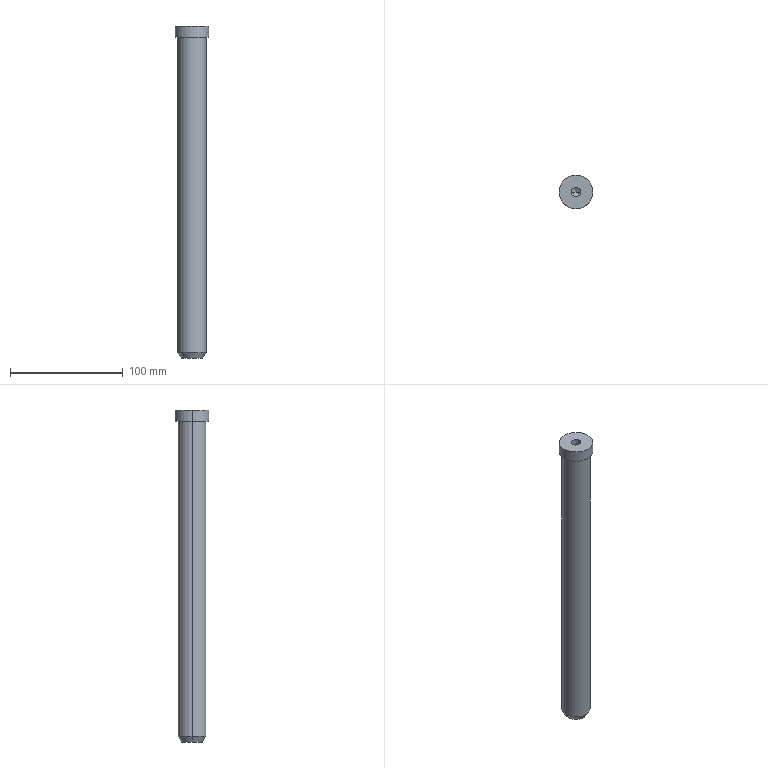Part | Creo | 1 solid | 13 faces | box 30 x 30 x 295 mm | volume 145243 mm3 | cylinder 6 | cone 4 | plane 3 | commonest cylinder face diameters 8.5 x2 25 x2 30 x2
STEP:
#1=CARTESIAN_POINT('',(0.,0.,0.));
#2=DIRECTION('',(0.,0.,1.));
#3=DIRECTION('',(1.,0.,0.));
#4=AXIS2_PLACEMENT_3D('',#1,#2,#3);
#5=CARTESIAN_POINT('',(-153.,131.,300.5));
#6=VERTEX_POINT('',#5);
#7=CARTESIAN_POINT('',(-123.,131.,300.5));
#8=VERTEX_POINT('',#7);
#9=CARTESIAN_POINT('',(-138.,131.,300.5));
#10=DIRECTION('',(0.,0.,-1.));
#11=DIRECTION('',(-1.,0.,0.));
#12=AXIS2_PLACEMENT_3D('',#9,#10,#11);
#13=CIRCLE('',#12,15.);
#14=EDGE_CURVE('',#6,#8,#13,.T.);
#15=ORIENTED_EDGE('',*,*,#14,.F.);
#16=CARTESIAN_POINT('',(-138.,131.,300.5));
#17=DIRECTION('',(0.,0.,-1.));
#18=DIRECTION('',(1.,0.,0.));
#19=AXIS2_PLACEMENT_3D('',#16,#17,#18);
#20=CIRCLE('',#19,15.);
#21=EDGE_CURVE('',#8,#6,#20,.T.);
#22=ORIENTED_EDGE('',*,*,#21,.F.);
#23=EDGE_LOOP('',(#15,#22));
#24=FACE_OUTER_BOUND('',#23,.F.);
#25=CARTESIAN_POINT('',(-150.5,131.,300.5));
#26=VERTEX_POINT('',#25);
#27=CARTESIAN_POINT('',(-125.5,131.,300.5));
#28=VERTEX_POINT('',#27);
#29=CARTESIAN_POINT('',(-138.,131.,300.5));
#30=DIRECTION('',(0.,0.,1.));
#31=DIRECTION('',(-1.,0.,0.));
#32=AXIS2_PLACEMENT_3D('',#29,#30,#31);
#33=CIRCLE('',#32,12.5);
#34=EDGE_CURVE('',#26,#28,#33,.T.);
#35=ORIENTED_EDGE('',*,*,#34,.F.);
#36=CARTESIAN_POINT('',(-138.,131.,300.5));
#37=DIRECTION('',(0.,0.,1.));
#38=DIRECTION('',(1.,0.,0.));
#39=AXIS2_PLACEMENT_3D('',#36,#37,#38);
#40=CIRCLE('',#39,12.5);
#41=EDGE_CURVE('',#28,#26,#40,.T.);
#42=ORIENTED_EDGE('',*,*,#41,.F.);
#43=EDGE_LOOP('',(#35,#42));
#44=FACE_BOUND('',#43,.F.);
#45=CARTESIAN_POINT('',(-138.,131.,300.5));
#46=DIRECTION('',(0.,0.,-1.));
#47=DIRECTION('',(-1.,0.,0.));
#48=AXIS2_PLACEMENT_3D('',#45,#46,#47);
#49=PLANE('',#48);
#50=ADVANCED_FACE('',(#24,#44),#49,.T.);
#51=CARTESIAN_POINT('',(-125.5,131.,20.5));
#52=VERTEX_POINT('',#51);
#53=CARTESIAN_POINT('',(-150.5,131.,20.5));
#54=VERTEX_POINT('',#53);
#55=CARTESIAN_POINT('',(-138.,131.,20.5));
#56=DIRECTION('',(0.,0.,-1.));
#57=DIRECTION('',(1.,0.,0.));
#58=AXIS2_PLACEMENT_3D('',#55,#56,#57);
#59=CIRCLE('',#58,12.5);
#60=EDGE_CURVE('',#52,#54,#59,.T.);
#61=ORIENTED_EDGE('',*,*,#60,.T.);
#62=CARTESIAN_POINT('',(-150.5,131.,20.5));
#63=DIRECTION('',(0.,0.,1.));
#64=VECTOR('',#63,280.);
#65=LINE('',#62,#64);
#66=EDGE_CURVE('',#54,#26,#65,.T.);
#67=ORIENTED_EDGE('',*,*,#66,.T.);
#68=ORIENTED_EDGE('',*,*,#34,.T.);
#69=CARTESIAN_POINT('',(-125.5,131.,20.5));
#70=DIRECTION('',(0.,0.,1.));
#71=VECTOR('',#70,280.);
#72=LINE('',#69,#71);
#73=EDGE_CURVE('',#52,#28,#72,.T.);
#74=ORIENTED_EDGE('',*,*,#73,.F.);
#75=EDGE_LOOP('',(#61,#67,#68,#74));
#76=FACE_OUTER_BOUND('',#75,.F.);
#77=CARTESIAN_POINT('',(-138.,131.,10.5));
#78=DIRECTION('',(0.,0.,1.));
#79=DIRECTION('',(1.,0.,0.));
#80=AXIS2_PLACEMENT_3D('',#77,#78,#79);
#81=CYLINDRICAL_SURFACE('',#80,12.5);
#82=ADVANCED_FACE('',(#76),#81,.T.);
#83=CARTESIAN_POINT('',(-128.5,131.,15.5));
#84=VERTEX_POINT('',#83);
#85=CARTESIAN_POINT('',(-147.5,131.,15.5));
#86=VERTEX_POINT('',#85);
#87=CARTESIAN_POINT('',(-138.,131.,15.5));
#88=DIRECTION('',(0.,0.,-1.));
#89=DIRECTION('',(1.,0.,0.));
#90=AXIS2_PLACEMENT_3D('',#87,#88,#89);
#91=CIRCLE('',#90,9.5);
#92=EDGE_CURVE('',#84,#86,#91,.T.);
#93=ORIENTED_EDGE('',*,*,#92,.T.);
#94=CARTESIAN_POINT('',(-147.5,131.,15.5));
#95=DIRECTION('',(-0.5145,0.,0.8575));
#96=VECTOR('',#95,5.831);
#97=LINE('',#94,#96);
#98=EDGE_CURVE('',#86,#54,#97,.T.);
#99=ORIENTED_EDGE('',*,*,#98,.T.);
#100=ORIENTED_EDGE('',*,*,#60,.F.);
#101=CARTESIAN_POINT('',(-128.5,131.,15.5));
#102=DIRECTION('',(0.5145,0.,0.8575));
#103=VECTOR('',#102,5.831);
#104=LINE('',#101,#103);
#105=EDGE_CURVE('',#84,#52,#104,.T.);
#106=ORIENTED_EDGE('',*,*,#105,.F.);
#107=EDGE_LOOP('',(#93,#99,#100,#106));
#108=FACE_OUTER_BOUND('',#107,.F.);
#109=CARTESIAN_POINT('',(-138.,131.,18.));
#110=DIRECTION('',(0.,0.,1.));
#111=DIRECTION('',(1.,0.,0.));
#112=AXIS2_PLACEMENT_3D('',#109,#110,#111);
#113=CONICAL_SURFACE('',#112,11.,30.964);
#114=ADVANCED_FACE('',(#108),#113,.T.);
#115=ORIENTED_EDGE('',*,*,#92,.F.);
#116=CARTESIAN_POINT('',(-138.,131.,15.5));
#117=DIRECTION('',(0.,0.,-1.));
#118=DIRECTION('',(-1.,0.,0.));
#119=AXIS2_PLACEMENT_3D('',#116,#117,#118);
#120=CIRCLE('',#119,9.5);
#121=EDGE_CURVE('',#86,#84,#120,.T.);
#122=ORIENTED_EDGE('',*,*,#121,.F.);
#123=EDGE_LOOP('',(#115,#122));
#124=FACE_OUTER_BOUND('',#123,.F.);
#125=CARTESIAN_POINT('',(-138.,131.,15.5));
#126=DIRECTION('',(0.,0.,1.));
#127=DIRECTION('',(1.,0.,0.));
#128=AXIS2_PLACEMENT_3D('',#125,#126,#127);
#129=PLANE('',#128);
#130=ADVANCED_FACE('',(#124),#129,.F.);
#131=ORIENTED_EDGE('',*,*,#121,.T.);
#132=ORIENTED_EDGE('',*,*,#105,.T.);
#133=CARTESIAN_POINT('',(-138.,131.,20.5));
#134=DIRECTION('',(0.,0.,-1.));
#135=DIRECTION('',(-1.,0.,0.));
#136=AXIS2_PLACEMENT_3D('',#133,#134,#135);
#137=CIRCLE('',#136,12.5);
#138=EDGE_CURVE('',#54,#52,#137,.T.);
#139=ORIENTED_EDGE('',*,*,#138,.F.);
#140=ORIENTED_EDGE('',*,*,#98,.F.);
#141=EDGE_LOOP('',(#131,#132,#139,#140));
#142=FACE_OUTER_BOUND('',#141,.F.);
#143=CARTESIAN_POINT('',(-138.,131.,18.));
#144=DIRECTION('',(0.,0.,1.));
#145=DIRECTION('',(1.,0.,0.));
#146=AXIS2_PLACEMENT_3D('',#143,#144,#145);
#147=CONICAL_SURFACE('',#146,11.,30.964);
#148=ADVANCED_FACE('',(#142),#147,.T.);
#149=ORIENTED_EDGE('',*,*,#138,.T.);
#150=ORIENTED_EDGE('',*,*,#73,.T.);
#151=ORIENTED_EDGE('',*,*,#41,.T.);
#152=ORIENTED_EDGE('',*,*,#66,.F.);
#153=EDGE_LOOP('',(#149,#150,#151,#152));
#154=FACE_OUTER_BOUND('',#153,.F.);
#155=CARTESIAN_POINT('',(-138.,131.,10.5));
#156=DIRECTION('',(0.,0.,1.));
#157=DIRECTION('',(1.,0.,0.));
#158=AXIS2_PLACEMENT_3D('',#155,#156,#157);
#159=CYLINDRICAL_SURFACE('',#158,12.5);
#160=ADVANCED_FACE('',(#154),#159,.T.);
#161=ORIENTED_EDGE('',*,*,#14,.T.);
#162=CARTESIAN_POINT('',(-123.,131.,310.5));
#163=VERTEX_POINT('',#162);
#164=CARTESIAN_POINT('',(-123.,131.,310.5));
#165=DIRECTION('',(0.,0.,-1.));
#166=VECTOR('',#165,10.);
#167=LINE('',#164,#166);
#168=EDGE_CURVE('',#163,#8,#167,.T.);
#169=ORIENTED_EDGE('',*,*,#168,.F.);
#170=CARTESIAN_POINT('',(-153.,131.,310.5));
#171=VERTEX_POINT('',#170);
#172=CARTESIAN_POINT('',(-138.,131.,310.5));
#173=DIRECTION('',(0.,0.,1.));
#174=DIRECTION('',(1.,0.,0.));
#175=AXIS2_PLACEMENT_3D('',#172,#173,#174);
#176=CIRCLE('',#175,15.);
#177=EDGE_CURVE('',#163,#171,#176,.T.);
#178=ORIENTED_EDGE('',*,*,#177,.T.);
#179=CARTESIAN_POINT('',(-153.,131.,310.5));
#180=DIRECTION('',(0.,0.,-1.));
#181=VECTOR('',#180,10.);
#182=LINE('',#179,#181);
#183=EDGE_CURVE('',#171,#6,#182,.T.);
#184=ORIENTED_EDGE('',*,*,#183,.T.);
#185=EDGE_LOOP('',(#161,#169,#178,#184));
#186=FACE_OUTER_BOUND('',#185,.F.);
#187=CARTESIAN_POINT('',(-138.,131.,310.5));
#188=DIRECTION('',(0.,0.,-1.));
#189=DIRECTION('',(-1.,0.,0.));
#190=AXIS2_PLACEMENT_3D('',#187,#188,#189);
#191=CYLINDRICAL_SURFACE('',#190,15.);
#192=ADVANCED_FACE('',(#186),#191,.T.);
#193=ORIENTED_EDGE('',*,*,#21,.T.);
#194=ORIENTED_EDGE('',*,*,#183,.F.);
#195=CARTESIAN_POINT('',(-138.,131.,310.5));
#196=DIRECTION('',(0.,0.,1.));
#197=DIRECTION('',(-1.,0.,0.));
#198=AXIS2_PLACEMENT_3D('',#195,#196,#197);
#199=CIRCLE('',#198,15.);
#200=EDGE_CURVE('',#171,#163,#199,.T.);
#201=ORIENTED_EDGE('',*,*,#200,.T.);
#202=ORIENTED_EDGE('',*,*,#168,.T.);
#203=EDGE_LOOP('',(#193,#194,#201,#202));
#204=FACE_OUTER_BOUND('',#203,.F.);
#205=CARTESIAN_POINT('',(-138.,131.,310.5));
#206=DIRECTION('',(0.,0.,-1.));
#207=DIRECTION('',(-1.,0.,0.));
#208=AXIS2_PLACEMENT_3D('',#205,#206,#207);
#209=CYLINDRICAL_SURFACE('',#208,15.);
#210=ADVANCED_FACE('',(#204),#209,.T.);
#211=ORIENTED_EDGE('',*,*,#200,.F.);
#212=ORIENTED_EDGE('',*,*,#177,.F.);
#213=EDGE_LOOP('',(#211,#212));
#214=FACE_OUTER_BOUND('',#213,.F.);
#215=CARTESIAN_POINT('',(-142.25,131.,310.5));
#216=VERTEX_POINT('',#215);
#217=CARTESIAN_POINT('',(-133.75,131.,310.5));
#218=VERTEX_POINT('',#217);
#219=CARTESIAN_POINT('',(-138.,131.,310.5));
#220=DIRECTION('',(0.,0.,-1.));
#221=DIRECTION('',(-1.,0.,0.));
#222=AXIS2_PLACEMENT_3D('',#219,#220,#221);
#223=CIRCLE('',#222,4.25);
#224=EDGE_CURVE('',#216,#218,#223,.T.);
#225=ORIENTED_EDGE('',*,*,#224,.F.);
#226=CARTESIAN_POINT('',(-138.,131.,310.5));
#227=DIRECTION('',(0.,0.,-1.));
#228=DIRECTION('',(1.,0.,0.));
#229=AXIS2_PLACEMENT_3D('',#226,#227,#228);
#230=CIRCLE('',#229,4.25);
#231=EDGE_CURVE('',#218,#216,#230,.T.);
#232=ORIENTED_EDGE('',*,*,#231,.F.);
#233=EDGE_LOOP('',(#225,#232));
#234=FACE_BOUND('',#233,.F.);
#235=CARTESIAN_POINT('',(-138.,131.,310.5));
#236=DIRECTION('',(0.,0.,1.));
#237=DIRECTION('',(1.,0.,0.));
#238=AXIS2_PLACEMENT_3D('',#235,#236,#237);
#239=PLANE('',#238);
#240=ADVANCED_FACE('',(#214,#234),#239,.T.);
#241=CARTESIAN_POINT('',(-133.75,131.,290.5));
#242=VERTEX_POINT('',#241);
#243=CARTESIAN_POINT('',(-142.25,131.,290.5));
#244=VERTEX_POINT('',#243);
#245=CARTESIAN_POINT('',(-138.,131.,290.5));
#246=DIRECTION('',(0.,0.,1.));
#247=DIRECTION('',(1.,0.,0.));
#248=AXIS2_PLACEMENT_3D('',#245,#246,#247);
#249=CIRCLE('',#248,4.25);
#250=EDGE_CURVE('',#242,#244,#249,.T.);
#251=ORIENTED_EDGE('',*,*,#250,.T.);
#252=CARTESIAN_POINT('',(-142.25,131.,310.5));
#253=DIRECTION('',(0.,0.,-1.));
#254=VECTOR('',#253,20.);
#255=LINE('',#252,#254);
#256=EDGE_CURVE('',#216,#244,#255,.T.);
#257=ORIENTED_EDGE('',*,*,#256,.F.);
#258=ORIENTED_EDGE('',*,*,#224,.T.);
#259=CARTESIAN_POINT('',(-133.75,131.,310.5));
#260=DIRECTION('',(0.,0.,-1.));
#261=VECTOR('',#260,20.);
#262=LINE('',#259,#261);
#263=EDGE_CURVE('',#218,#242,#262,.T.);
#264=ORIENTED_EDGE('',*,*,#263,.T.);
#265=EDGE_LOOP('',(#251,#257,#258,#264));
#266=FACE_OUTER_BOUND('',#265,.F.);
#267=CARTESIAN_POINT('',(-138.,131.,310.5));
#268=DIRECTION('',(0.,0.,-1.));
#269=DIRECTION('',(-1.,0.,0.));
#270=AXIS2_PLACEMENT_3D('',#267,#268,#269);
#271=CYLINDRICAL_SURFACE('',#270,4.25);
#272=ADVANCED_FACE('',(#266),#271,.F.);
#273=ORIENTED_EDGE('',*,*,#250,.F.);
#274=CARTESIAN_POINT('',(-138.,131.,287.946));
#275=VERTEX_POINT('',#274);
#276=CARTESIAN_POINT('',(-138.,131.,287.946));
#277=DIRECTION('',(0.8572,0.,0.515));
#278=VECTOR('',#277,4.958);
#279=LINE('',#276,#278);
#280=EDGE_CURVE('',#275,#242,#279,.T.);
#281=ORIENTED_EDGE('',*,*,#280,.F.);
#282=CARTESIAN_POINT('',(-138.,131.,287.946));
#283=DIRECTION('',(-0.8572,0.,0.515));
#284=VECTOR('',#283,4.958);
#285=LINE('',#282,#284);
#286=EDGE_CURVE('',#275,#244,#285,.T.);
#287=ORIENTED_EDGE('',*,*,#286,.T.);
#288=EDGE_LOOP('',(#273,#281,#287));
#289=FACE_OUTER_BOUND('',#288,.F.);
#290=CARTESIAN_POINT('',(-138.,131.,289.315));
#291=DIRECTION('',(0.,0.,1.));
#292=DIRECTION('',(1.,0.,0.));
#293=AXIS2_PLACEMENT_3D('',#290,#291,#292);
#294=CONICAL_SURFACE('',#293,2.278,59.);
#295=ADVANCED_FACE('',(#289),#294,.F.);
#296=CARTESIAN_POINT('',(-138.,131.,290.5));
#297=DIRECTION('',(0.,0.,1.));
#298=DIRECTION('',(-1.,0.,0.));
#299=AXIS2_PLACEMENT_3D('',#296,#297,#298);
#300=CIRCLE('',#299,4.25);
#301=EDGE_CURVE('',#244,#242,#300,.T.);
#302=ORIENTED_EDGE('',*,*,#301,.F.);
#303=ORIENTED_EDGE('',*,*,#286,.F.);
#304=ORIENTED_EDGE('',*,*,#280,.T.);
#305=EDGE_LOOP('',(#302,#303,#304));
#306=FACE_OUTER_BOUND('',#305,.F.);
#307=CARTESIAN_POINT('',(-138.,131.,289.315));
#308=DIRECTION('',(0.,0.,1.));
#309=DIRECTION('',(1.,0.,0.));
#310=AXIS2_PLACEMENT_3D('',#307,#308,#309);
#311=CONICAL_SURFACE('',#310,2.278,59.);
#312=ADVANCED_FACE('',(#306),#311,.F.);
#313=ORIENTED_EDGE('',*,*,#301,.T.);
#314=ORIENTED_EDGE('',*,*,#263,.F.);
#315=ORIENTED_EDGE('',*,*,#231,.T.);
#316=ORIENTED_EDGE('',*,*,#256,.T.);
#317=EDGE_LOOP('',(#313,#314,#315,#316));
#318=FACE_OUTER_BOUND('',#317,.F.);
#319=CARTESIAN_POINT('',(-138.,131.,310.5));
#320=DIRECTION('',(0.,0.,-1.));
#321=DIRECTION('',(-1.,0.,0.));
#322=AXIS2_PLACEMENT_3D('',#319,#320,#321);
#323=CYLINDRICAL_SURFACE('',#322,4.25);
#324=ADVANCED_FACE('',(#318),#323,.F.);
#325=CLOSED_SHELL('',(#50,#82,#114,#130,#148,#160,#192,#210,#240,#272,#295,#312,#324));
#326=MANIFOLD_SOLID_BREP('',#325);
#327=(LENGTH_UNIT()NAMED_UNIT(*)SI_UNIT(.MILLI.,.METRE.));
#328=UNCERTAINTY_MEASURE_WITH_UNIT(LENGTH_MEASURE(0.0298),#327,'','');
#329=(NAMED_UNIT(*)PLANE_ANGLE_UNIT()SI_UNIT($,.RADIAN.));
#330=PLANE_ANGLE_MEASURE_WITH_UNIT(PLANE_ANGLE_MEASURE(0.01745),#329);
#331=(CONVERSION_BASED_UNIT('DEGREE',#330)NAMED_UNIT(*)PLANE_ANGLE_UNIT());
#332=(NAMED_UNIT(*)SI_UNIT($,.STERADIAN.)SOLID_ANGLE_UNIT());
#333=(GEOMETRIC_REPRESENTATION_CONTEXT(3)GLOBAL_UNCERTAINTY_ASSIGNED_CONTEXT((#328))GLOBAL_UNIT_ASSIGNED_CONTEXT((#327,#331,#332))REPRESENTATION_CONTEXT('',''));
#334=ADVANCED_BREP_SHAPE_REPRESENTATION('',(#4,#326),#333);